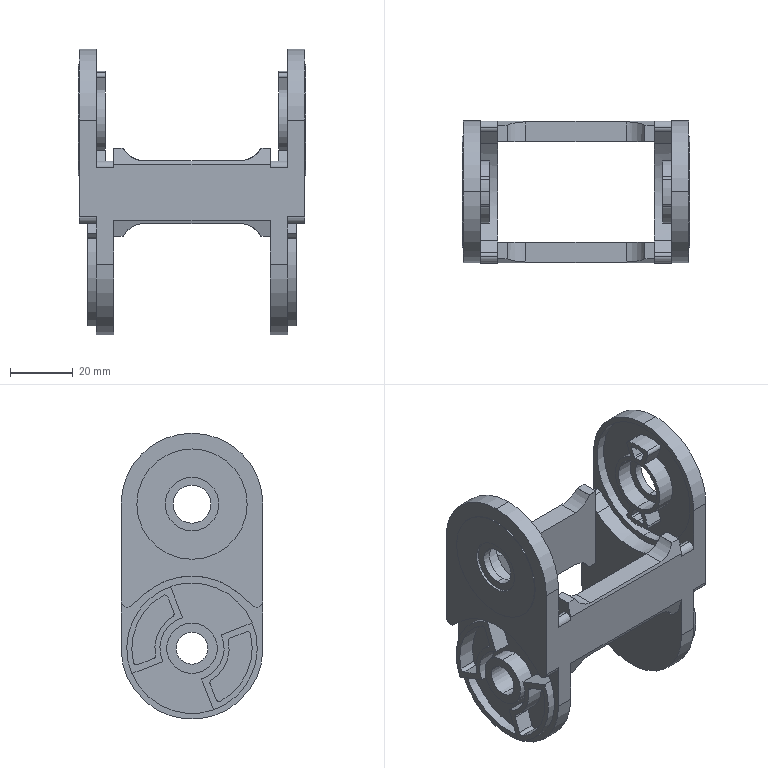Part | SolidWorks | features BaseBody 1 | 1 solid | 262 faces | box 72.6 x 45.28 x 91.28 mm | volume 47406 mm3 | cylinder 164 | plane 98 | commonest cylinder face diameters 2 x28 1 x20 4 x12 20.12 x10 41.64 x10 0.2 x8